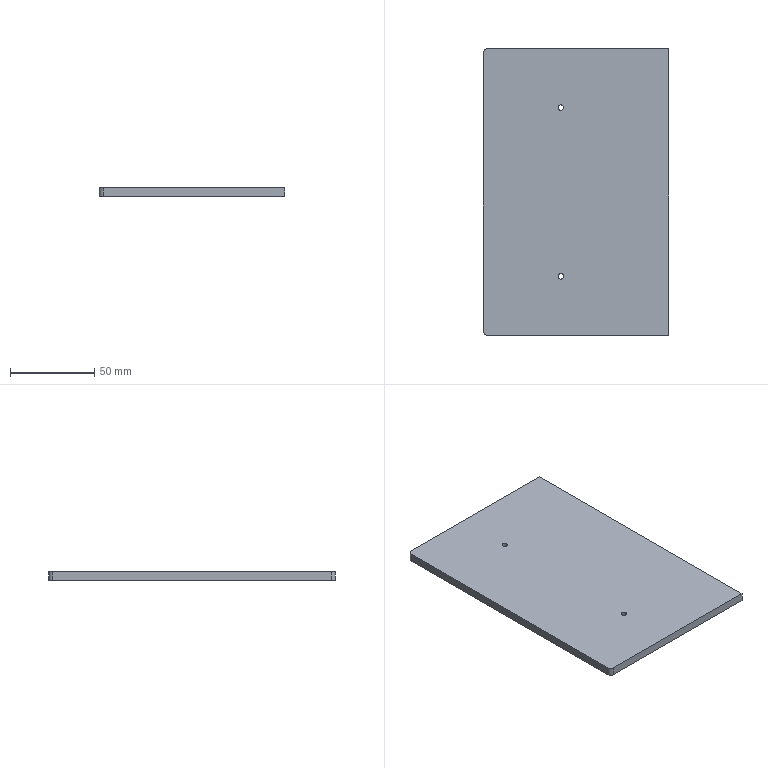Part | NX | features BREP 1 | 1 solid | 10 faces | box 110 x 170 x 5 mm | volume 93401 mm3 | plane 6 | cylinder 4 | commonest cylinder face diameters 3.3 x2 5 x2
STEP:
#1=CARTESIAN_POINT('',(-7.35,-50.,0.));
#2=VERTEX_POINT('',#1);
#3=CARTESIAN_POINT('',(-9.,-50.,0.));
#4=DIRECTION('',(0.,0.,1.));
#5=DIRECTION('',(1.,0.,0.));
#6=AXIS2_PLACEMENT_3D('',#3,#4,#5);
#7=CIRCLE('',#6,1.65);
#8=EDGE_CURVE('',#2,#2,#7,.T.);
#9=ORIENTED_EDGE('',*,*,#8,.T.);
#10=EDGE_LOOP('',(#9));
#11=FACE_BOUND('',#10,.T.);
#12=CARTESIAN_POINT('',(-7.35,-50.,-5.));
#13=VERTEX_POINT('',#12);
#14=CARTESIAN_POINT('',(-9.,-50.,-5.));
#15=DIRECTION('',(0.,0.,1.));
#16=DIRECTION('',(1.,0.,0.));
#17=AXIS2_PLACEMENT_3D('',#14,#15,#16);
#18=CIRCLE('',#17,1.65);
#19=EDGE_CURVE('',#13,#13,#18,.T.);
#20=ORIENTED_EDGE('',*,*,#19,.F.);
#21=EDGE_LOOP('',(#20));
#22=FACE_BOUND('',#21,.T.);
#23=CARTESIAN_POINT('',(-9.,-50.,0.));
#24=DIRECTION('',(0.,0.,1.));
#25=DIRECTION('',(1.,0.,0.));
#26=AXIS2_PLACEMENT_3D('',#23,#24,#25);
#27=CYLINDRICAL_SURFACE('',#26,1.65);
#28=ADVANCED_FACE('',(#11,#22),#27,.F.);
#29=CARTESIAN_POINT('',(-7.35,50.,0.));
#30=VERTEX_POINT('',#29);
#31=CARTESIAN_POINT('',(-9.,50.,0.));
#32=DIRECTION('',(0.,0.,1.));
#33=DIRECTION('',(1.,0.,0.));
#34=AXIS2_PLACEMENT_3D('',#31,#32,#33);
#35=CIRCLE('',#34,1.65);
#36=EDGE_CURVE('',#30,#30,#35,.T.);
#37=ORIENTED_EDGE('',*,*,#36,.T.);
#38=EDGE_LOOP('',(#37));
#39=FACE_BOUND('',#38,.T.);
#40=CARTESIAN_POINT('',(-7.35,50.,-5.));
#41=VERTEX_POINT('',#40);
#42=CARTESIAN_POINT('',(-9.,50.,-5.));
#43=DIRECTION('',(0.,0.,1.));
#44=DIRECTION('',(1.,0.,0.));
#45=AXIS2_PLACEMENT_3D('',#42,#43,#44);
#46=CIRCLE('',#45,1.65);
#47=EDGE_CURVE('',#41,#41,#46,.T.);
#48=ORIENTED_EDGE('',*,*,#47,.F.);
#49=EDGE_LOOP('',(#48));
#50=FACE_BOUND('',#49,.T.);
#51=CARTESIAN_POINT('',(-9.,50.,0.));
#52=DIRECTION('',(0.,0.,1.));
#53=DIRECTION('',(1.,0.,0.));
#54=AXIS2_PLACEMENT_3D('',#51,#52,#53);
#55=CYLINDRICAL_SURFACE('',#54,1.65);
#56=ADVANCED_FACE('',(#39,#50),#55,.F.);
#57=CARTESIAN_POINT('',(55.,-85.,0.));
#58=VERTEX_POINT('',#57);
#59=CARTESIAN_POINT('',(55.,85.,0.));
#60=VERTEX_POINT('',#59);
#61=CARTESIAN_POINT('',(55.,-85.,0.));
#62=DIRECTION('',(0.,1.,0.));
#63=VECTOR('',#62,1000.);
#64=LINE('',#61,#63);
#65=EDGE_CURVE('',#58,#60,#64,.T.);
#66=ORIENTED_EDGE('',*,*,#65,.F.);
#67=CARTESIAN_POINT('',(55.,-85.,-5.));
#68=VERTEX_POINT('',#67);
#69=CARTESIAN_POINT('',(55.,-85.,-5.));
#70=DIRECTION('',(0.,0.,1.));
#71=VECTOR('',#70,1000.);
#72=LINE('',#69,#71);
#73=EDGE_CURVE('',#68,#58,#72,.T.);
#74=ORIENTED_EDGE('',*,*,#73,.F.);
#75=CARTESIAN_POINT('',(55.,85.,-5.));
#76=VERTEX_POINT('',#75);
#77=CARTESIAN_POINT('',(55.,-85.,-5.));
#78=DIRECTION('',(0.,1.,0.));
#79=VECTOR('',#78,1000.);
#80=LINE('',#77,#79);
#81=EDGE_CURVE('',#68,#76,#80,.T.);
#82=ORIENTED_EDGE('',*,*,#81,.T.);
#83=CARTESIAN_POINT('',(55.,85.,-5.));
#84=DIRECTION('',(0.,0.,1.));
#85=VECTOR('',#84,1000.);
#86=LINE('',#83,#85);
#87=EDGE_CURVE('',#76,#60,#86,.T.);
#88=ORIENTED_EDGE('',*,*,#87,.T.);
#89=EDGE_LOOP('',(#66,#74,#82,#88));
#90=FACE_BOUND('',#89,.T.);
#91=CARTESIAN_POINT('',(55.,-85.,-5.));
#92=DIRECTION('',(1.,0.,0.));
#93=DIRECTION('',(0.,0.,-1.));
#94=AXIS2_PLACEMENT_3D('',#91,#92,#93);
#95=PLANE('',#94);
#96=ADVANCED_FACE('',(#90),#95,.T.);
#97=CARTESIAN_POINT('',(-52.5,-85.,0.));
#98=VERTEX_POINT('',#97);
#99=CARTESIAN_POINT('',(-55.,-85.,0.));
#100=DIRECTION('',(1.,0.,0.));
#101=VECTOR('',#100,1000.);
#102=LINE('',#99,#101);
#103=EDGE_CURVE('',#98,#58,#102,.T.);
#104=ORIENTED_EDGE('',*,*,#103,.F.);
#105=CARTESIAN_POINT('',(-52.5,-85.,-5.));
#106=VERTEX_POINT('',#105);
#107=CARTESIAN_POINT('',(-52.5,-85.,-5.));
#108=DIRECTION('',(0.,0.,-1.));
#109=VECTOR('',#108,1000.);
#110=LINE('',#107,#109);
#111=EDGE_CURVE('',#98,#106,#110,.T.);
#112=ORIENTED_EDGE('',*,*,#111,.T.);
#113=CARTESIAN_POINT('',(-55.,-85.,-5.));
#114=DIRECTION('',(1.,0.,0.));
#115=VECTOR('',#114,1000.);
#116=LINE('',#113,#115);
#117=EDGE_CURVE('',#106,#68,#116,.T.);
#118=ORIENTED_EDGE('',*,*,#117,.T.);
#119=ORIENTED_EDGE('',*,*,#73,.T.);
#120=EDGE_LOOP('',(#104,#112,#118,#119));
#121=FACE_BOUND('',#120,.T.);
#122=CARTESIAN_POINT('',(-55.,-85.,-5.));
#123=DIRECTION('',(0.,-1.,0.));
#124=DIRECTION('',(0.,0.,-1.));
#125=AXIS2_PLACEMENT_3D('',#122,#123,#124);
#126=PLANE('',#125);
#127=ADVANCED_FACE('',(#121),#126,.T.);
#128=CARTESIAN_POINT('',(-55.,82.5,-5.));
#129=VERTEX_POINT('',#128);
#130=CARTESIAN_POINT('',(-55.,-82.5,-5.));
#131=VERTEX_POINT('',#130);
#132=CARTESIAN_POINT('',(-55.,-85.,-5.));
#133=DIRECTION('',(0.,-1.,0.));
#134=VECTOR('',#133,1000.);
#135=LINE('',#132,#134);
#136=EDGE_CURVE('',#129,#131,#135,.T.);
#137=ORIENTED_EDGE('',*,*,#136,.T.);
#138=CARTESIAN_POINT('',(-55.,-82.5,0.));
#139=VERTEX_POINT('',#138);
#140=CARTESIAN_POINT('',(-55.,-82.5,-5.));
#141=DIRECTION('',(0.,0.,1.));
#142=VECTOR('',#141,1000.);
#143=LINE('',#140,#142);
#144=EDGE_CURVE('',#131,#139,#143,.T.);
#145=ORIENTED_EDGE('',*,*,#144,.T.);
#146=CARTESIAN_POINT('',(-55.,82.5,0.));
#147=VERTEX_POINT('',#146);
#148=CARTESIAN_POINT('',(-55.,-85.,0.));
#149=DIRECTION('',(0.,-1.,0.));
#150=VECTOR('',#149,1000.);
#151=LINE('',#148,#150);
#152=EDGE_CURVE('',#147,#139,#151,.T.);
#153=ORIENTED_EDGE('',*,*,#152,.F.);
#154=CARTESIAN_POINT('',(-55.,82.5,-5.));
#155=DIRECTION('',(0.,0.,-1.));
#156=VECTOR('',#155,1000.);
#157=LINE('',#154,#156);
#158=EDGE_CURVE('',#147,#129,#157,.T.);
#159=ORIENTED_EDGE('',*,*,#158,.T.);
#160=EDGE_LOOP('',(#137,#145,#153,#159));
#161=FACE_BOUND('',#160,.T.);
#162=CARTESIAN_POINT('',(-55.,-85.,-5.));
#163=DIRECTION('',(-1.,0.,0.));
#164=DIRECTION('',(0.,0.,1.));
#165=AXIS2_PLACEMENT_3D('',#162,#163,#164);
#166=PLANE('',#165);
#167=ADVANCED_FACE('',(#161),#166,.T.);
#168=CARTESIAN_POINT('',(-52.5,85.,-5.));
#169=VERTEX_POINT('',#168);
#170=CARTESIAN_POINT('',(-55.,85.,-5.));
#171=DIRECTION('',(-1.,0.,0.));
#172=VECTOR('',#171,1000.);
#173=LINE('',#170,#172);
#174=EDGE_CURVE('',#76,#169,#173,.T.);
#175=ORIENTED_EDGE('',*,*,#174,.T.);
#176=CARTESIAN_POINT('',(-52.5,85.,0.));
#177=VERTEX_POINT('',#176);
#178=CARTESIAN_POINT('',(-52.5,85.,-5.));
#179=DIRECTION('',(0.,0.,1.));
#180=VECTOR('',#179,1000.);
#181=LINE('',#178,#180);
#182=EDGE_CURVE('',#169,#177,#181,.T.);
#183=ORIENTED_EDGE('',*,*,#182,.T.);
#184=CARTESIAN_POINT('',(-55.,85.,0.));
#185=DIRECTION('',(-1.,0.,0.));
#186=VECTOR('',#185,1000.);
#187=LINE('',#184,#186);
#188=EDGE_CURVE('',#60,#177,#187,.T.);
#189=ORIENTED_EDGE('',*,*,#188,.F.);
#190=ORIENTED_EDGE('',*,*,#87,.F.);
#191=EDGE_LOOP('',(#175,#183,#189,#190));
#192=FACE_BOUND('',#191,.T.);
#193=CARTESIAN_POINT('',(-55.,85.,-5.));
#194=DIRECTION('',(0.,1.,0.));
#195=DIRECTION('',(0.,0.,1.));
#196=AXIS2_PLACEMENT_3D('',#193,#194,#195);
#197=PLANE('',#196);
#198=ADVANCED_FACE('',(#192),#197,.T.);
#199=ORIENTED_EDGE('',*,*,#19,.T.);
#200=EDGE_LOOP('',(#199));
#201=FACE_BOUND('',#200,.T.);
#202=ORIENTED_EDGE('',*,*,#47,.T.);
#203=EDGE_LOOP('',(#202));
#204=FACE_BOUND('',#203,.T.);
#205=ORIENTED_EDGE('',*,*,#117,.F.);
#206=CARTESIAN_POINT('',(-52.5,-82.5,-5.));
#207=DIRECTION('',(0.,0.,-1.));
#208=DIRECTION('',(-1.,0.,0.));
#209=AXIS2_PLACEMENT_3D('',#206,#207,#208);
#210=CIRCLE('',#209,2.5);
#211=EDGE_CURVE('',#106,#131,#210,.T.);
#212=ORIENTED_EDGE('',*,*,#211,.T.);
#213=ORIENTED_EDGE('',*,*,#136,.F.);
#214=CARTESIAN_POINT('',(-52.5,82.5,-5.));
#215=DIRECTION('',(0.,0.,-1.));
#216=DIRECTION('',(-1.,0.,0.));
#217=AXIS2_PLACEMENT_3D('',#214,#215,#216);
#218=CIRCLE('',#217,2.5);
#219=EDGE_CURVE('',#129,#169,#218,.T.);
#220=ORIENTED_EDGE('',*,*,#219,.T.);
#221=ORIENTED_EDGE('',*,*,#174,.F.);
#222=ORIENTED_EDGE('',*,*,#81,.F.);
#223=EDGE_LOOP('',(#205,#212,#213,#220,#221,#222));
#224=FACE_BOUND('',#223,.T.);
#225=CARTESIAN_POINT('',(0.,0.,-5.));
#226=DIRECTION('',(0.,0.,-1.));
#227=DIRECTION('',(-1.,0.,0.));
#228=AXIS2_PLACEMENT_3D('',#225,#226,#227);
#229=PLANE('',#228);
#230=ADVANCED_FACE('',(#201,#204,#224),#229,.T.);
#231=ORIENTED_EDGE('',*,*,#8,.F.);
#232=EDGE_LOOP('',(#231));
#233=FACE_BOUND('',#232,.T.);
#234=ORIENTED_EDGE('',*,*,#36,.F.);
#235=EDGE_LOOP('',(#234));
#236=FACE_BOUND('',#235,.T.);
#237=ORIENTED_EDGE('',*,*,#152,.T.);
#238=CARTESIAN_POINT('',(-52.5,-82.5,0.));
#239=DIRECTION('',(0.,0.,1.));
#240=DIRECTION('',(-1.,0.,0.));
#241=AXIS2_PLACEMENT_3D('',#238,#239,#240);
#242=CIRCLE('',#241,2.5);
#243=EDGE_CURVE('',#139,#98,#242,.T.);
#244=ORIENTED_EDGE('',*,*,#243,.T.);
#245=ORIENTED_EDGE('',*,*,#103,.T.);
#246=ORIENTED_EDGE('',*,*,#65,.T.);
#247=ORIENTED_EDGE('',*,*,#188,.T.);
#248=CARTESIAN_POINT('',(-52.5,82.5,0.));
#249=DIRECTION('',(0.,0.,1.));
#250=DIRECTION('',(-1.,0.,0.));
#251=AXIS2_PLACEMENT_3D('',#248,#249,#250);
#252=CIRCLE('',#251,2.5);
#253=EDGE_CURVE('',#177,#147,#252,.T.);
#254=ORIENTED_EDGE('',*,*,#253,.T.);
#255=EDGE_LOOP('',(#237,#244,#245,#246,#247,#254));
#256=FACE_BOUND('',#255,.T.);
#257=CARTESIAN_POINT('',(0.,0.,0.));
#258=DIRECTION('',(0.,0.,-1.));
#259=DIRECTION('',(-1.,0.,0.));
#260=AXIS2_PLACEMENT_3D('',#257,#258,#259);
#261=PLANE('',#260);
#262=ADVANCED_FACE('',(#233,#236,#256),#261,.F.);
#263=ORIENTED_EDGE('',*,*,#219,.F.);
#264=ORIENTED_EDGE('',*,*,#158,.F.);
#265=ORIENTED_EDGE('',*,*,#253,.F.);
#266=ORIENTED_EDGE('',*,*,#182,.F.);
#267=EDGE_LOOP('',(#263,#264,#265,#266));
#268=FACE_BOUND('',#267,.T.);
#269=CARTESIAN_POINT('',(-52.5,82.5,-5.));
#270=DIRECTION('',(0.,0.,1.));
#271=DIRECTION('',(1.,0.,0.));
#272=AXIS2_PLACEMENT_3D('',#269,#270,#271);
#273=CYLINDRICAL_SURFACE('',#272,2.5);
#274=ADVANCED_FACE('',(#268),#273,.T.);
#275=ORIENTED_EDGE('',*,*,#211,.F.);
#276=ORIENTED_EDGE('',*,*,#111,.F.);
#277=ORIENTED_EDGE('',*,*,#243,.F.);
#278=ORIENTED_EDGE('',*,*,#144,.F.);
#279=EDGE_LOOP('',(#275,#276,#277,#278));
#280=FACE_BOUND('',#279,.T.);
#281=CARTESIAN_POINT('',(-52.5,-82.5,-5.));
#282=DIRECTION('',(0.,0.,1.));
#283=DIRECTION('',(1.,0.,0.));
#284=AXIS2_PLACEMENT_3D('',#281,#282,#283);
#285=CYLINDRICAL_SURFACE('',#284,2.5);
#286=ADVANCED_FACE('',(#280),#285,.T.);
#287=CLOSED_SHELL('',(#28,#56,#96,#127,#167,#198,#230,#262,#274,#286));
#288=MANIFOLD_SOLID_BREP('',#287);
#289=(LENGTH_UNIT()NAMED_UNIT(*)SI_UNIT(.MILLI.,.METRE.));
#290=UNCERTAINTY_MEASURE_WITH_UNIT(LENGTH_MEASURE(0.00001),#289,'','');
#291=(NAMED_UNIT(*)PLANE_ANGLE_UNIT()SI_UNIT($,.RADIAN.));
#292=(NAMED_UNIT(*)SI_UNIT($,.STERADIAN.)SOLID_ANGLE_UNIT());
#293=(GEOMETRIC_REPRESENTATION_CONTEXT(3)GLOBAL_UNCERTAINTY_ASSIGNED_CONTEXT((#290))GLOBAL_UNIT_ASSIGNED_CONTEXT((#289,#291,#292))REPRESENTATION_CONTEXT('',''));
#294=ADVANCED_BREP_SHAPE_REPRESENTATION('',(#288),#293);